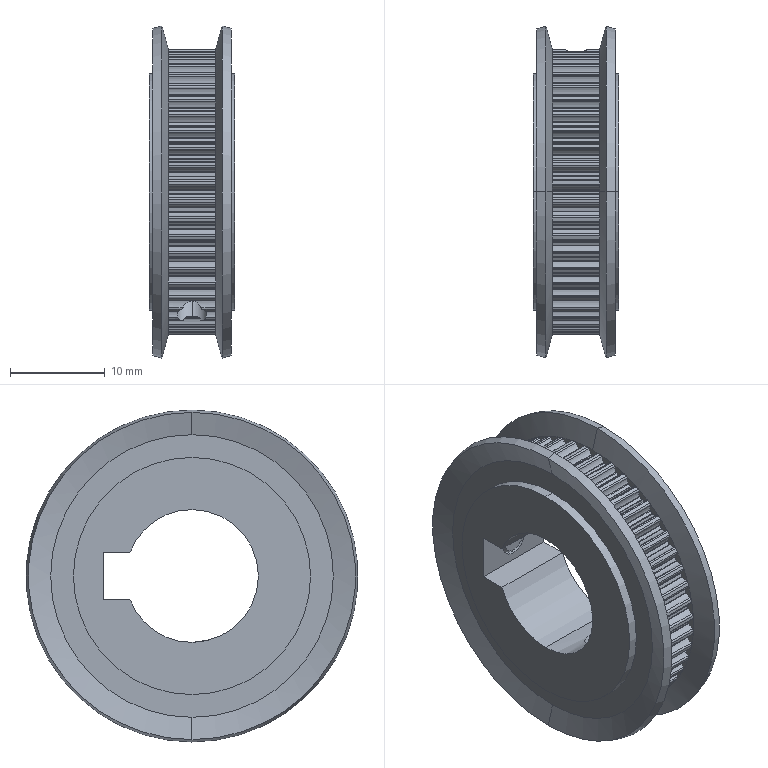Part | SolidWorks | 3 solids | 618 faces | box 9 x 35 x 35 mm | volume 4712 mm3 | cylinder 463 | plane 131 | cone 24 | commonest cylinder face diameters 0.38 x124 0.2 x113 2.65 x108 30.05 x52 28.53 x51 3.242 x4